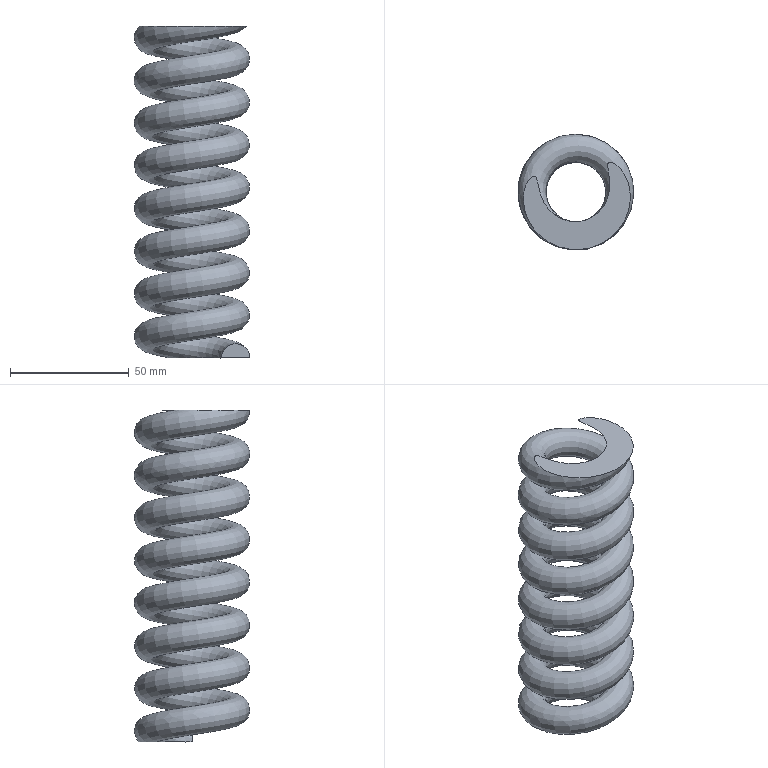Part | NX | features solid 2 | 1 solid | 4 faces | box 48.928 x 48.851 x 140 mm | volume 99028 mm3 | plane 3 | spline 1